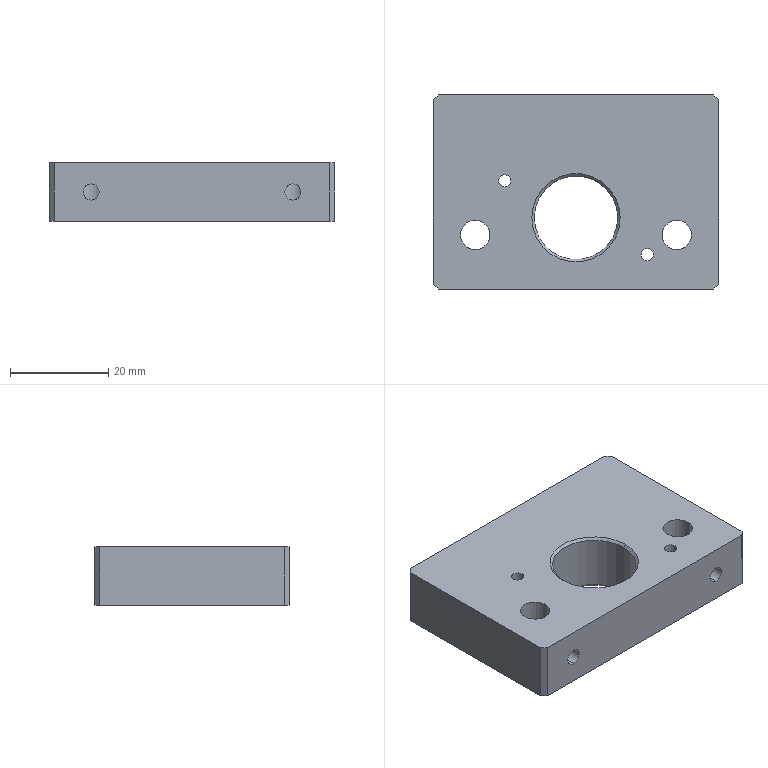Part | SolidWorks | features Chamfer 2, HoleWzd 2, Extrusion 1, MirrorPattern 1 | 1 solid | 36 faces | box 58 x 39.5 x 12 mm | volume 23617 mm3 | cylinder 18 | plane 10 | cone 8 | commonest cylinder face diameters 3.3 x8 2.5 x4 6 x4 17 x2
STEP:
#1=CARTESIAN_POINT('',(-8.5,-5.25,5.5));
#2=VERTEX_POINT('',#1);
#3=CARTESIAN_POINT('',(8.5,-5.25,5.5));
#4=VERTEX_POINT('',#3);
#5=CARTESIAN_POINT('',(0.,-5.25,5.5));
#6=DIRECTION('',(0.,0.,1.));
#7=DIRECTION('',(1.,0.,0.));
#8=AXIS2_PLACEMENT_3D('',#5,#6,#7);
#9=CIRCLE('',#8,8.5);
#10=EDGE_CURVE('',#2,#4,#9,.T.);
#11=ORIENTED_EDGE('',*,*,#10,.F.);
#12=CARTESIAN_POINT('',(-9.,-5.25,6.));
#13=VERTEX_POINT('',#12);
#14=CARTESIAN_POINT('',(-8.5,-5.25,5.5));
#15=DIRECTION('',(-0.7071,0.,0.7071));
#16=VECTOR('',#15,1000.);
#17=LINE('',#14,#16);
#18=EDGE_CURVE('',#2,#13,#17,.T.);
#19=ORIENTED_EDGE('',*,*,#18,.T.);
#20=CARTESIAN_POINT('',(9.,-5.25,6.));
#21=VERTEX_POINT('',#20);
#22=CARTESIAN_POINT('',(0.,-5.25,6.));
#23=DIRECTION('',(0.,0.,-1.));
#24=DIRECTION('',(1.,0.,0.));
#25=AXIS2_PLACEMENT_3D('',#22,#23,#24);
#26=CIRCLE('',#25,9.);
#27=EDGE_CURVE('',#21,#13,#26,.T.);
#28=ORIENTED_EDGE('',*,*,#27,.F.);
#29=CARTESIAN_POINT('',(8.5,-5.25,5.5));
#30=DIRECTION('',(0.7071,0.,0.7071));
#31=VECTOR('',#30,1000.);
#32=LINE('',#29,#31);
#33=EDGE_CURVE('',#4,#21,#32,.T.);
#34=ORIENTED_EDGE('',*,*,#33,.F.);
#35=EDGE_LOOP('',(#11,#19,#28,#34));
#36=FACE_OUTER_BOUND('',#35,.T.);
#37=CARTESIAN_POINT('',(0.,-5.25,5.5));
#38=DIRECTION('',(0.,0.,1.));
#39=DIRECTION('',(1.,0.,0.));
#40=AXIS2_PLACEMENT_3D('',#37,#38,#39);
#41=CONICAL_SURFACE('',#40,8.5,0.7854);
#42=ADVANCED_FACE('',(#36),#41,.F.);
#43=CARTESIAN_POINT('',(8.5,-5.25,-5.5));
#44=VERTEX_POINT('',#43);
#45=CARTESIAN_POINT('',(-8.5,-5.25,-5.5));
#46=VERTEX_POINT('',#45);
#47=CARTESIAN_POINT('',(0.,-5.25,-5.5));
#48=DIRECTION('',(0.,0.,-1.));
#49=DIRECTION('',(1.,0.,0.));
#50=AXIS2_PLACEMENT_3D('',#47,#48,#49);
#51=CIRCLE('',#50,8.5);
#52=EDGE_CURVE('',#44,#46,#51,.T.);
#53=ORIENTED_EDGE('',*,*,#52,.F.);
#54=CARTESIAN_POINT('',(9.,-5.25,-6.));
#55=VERTEX_POINT('',#54);
#56=CARTESIAN_POINT('',(9.,-5.25,-6.));
#57=DIRECTION('',(0.7071,0.,-0.7071));
#58=VECTOR('',#57,1000.);
#59=LINE('',#56,#58);
#60=EDGE_CURVE('',#44,#55,#59,.T.);
#61=ORIENTED_EDGE('',*,*,#60,.T.);
#62=CARTESIAN_POINT('',(-9.,-5.25,-6.));
#63=VERTEX_POINT('',#62);
#64=CARTESIAN_POINT('',(0.,-5.25,-6.));
#65=DIRECTION('',(0.,0.,1.));
#66=DIRECTION('',(1.,0.,0.));
#67=AXIS2_PLACEMENT_3D('',#64,#65,#66);
#68=CIRCLE('',#67,9.);
#69=EDGE_CURVE('',#63,#55,#68,.T.);
#70=ORIENTED_EDGE('',*,*,#69,.F.);
#71=CARTESIAN_POINT('',(-9.,-5.25,-6.));
#72=DIRECTION('',(-0.7071,0.,-0.7071));
#73=VECTOR('',#72,1000.);
#74=LINE('',#71,#73);
#75=EDGE_CURVE('',#46,#63,#74,.T.);
#76=ORIENTED_EDGE('',*,*,#75,.F.);
#77=EDGE_LOOP('',(#53,#61,#70,#76));
#78=FACE_OUTER_BOUND('',#77,.T.);
#79=CARTESIAN_POINT('',(0.,-5.25,-6.));
#80=DIRECTION('',(0.,0.,-1.));
#81=DIRECTION('',(-1.,0.,0.));
#82=AXIS2_PLACEMENT_3D('',#79,#80,#81);
#83=CONICAL_SURFACE('',#82,9.,0.7854);
#84=ADVANCED_FACE('',(#78),#83,.F.);
#85=CARTESIAN_POINT('',(-20.5,9.65,-1.65));
#86=VERTEX_POINT('',#85);
#87=CARTESIAN_POINT('',(-20.5,9.65,1.65));
#88=VERTEX_POINT('',#87);
#89=CARTESIAN_POINT('',(-20.5,9.65,0.));
#90=DIRECTION('',(0.,1.,0.));
#91=DIRECTION('',(0.,0.,1.));
#92=AXIS2_PLACEMENT_3D('',#89,#90,#91);
#93=CIRCLE('',#92,1.65);
#94=EDGE_CURVE('',#86,#88,#93,.T.);
#95=ORIENTED_EDGE('',*,*,#94,.F.);
#96=CARTESIAN_POINT('',(-20.5,19.75,-1.65));
#97=VERTEX_POINT('',#96);
#98=CARTESIAN_POINT('',(-20.5,19.75,-1.65));
#99=DIRECTION('',(0.,1.,0.));
#100=VECTOR('',#99,1000.);
#101=LINE('',#98,#100);
#102=EDGE_CURVE('',#86,#97,#101,.T.);
#103=ORIENTED_EDGE('',*,*,#102,.T.);
#104=CARTESIAN_POINT('',(-20.5,19.75,1.65));
#105=VERTEX_POINT('',#104);
#106=CARTESIAN_POINT('',(-20.5,19.75,0.));
#107=DIRECTION('',(0.,1.,0.));
#108=DIRECTION('',(0.,0.,1.));
#109=AXIS2_PLACEMENT_3D('',#106,#107,#108);
#110=CIRCLE('',#109,1.65);
#111=EDGE_CURVE('',#97,#105,#110,.T.);
#112=ORIENTED_EDGE('',*,*,#111,.T.);
#113=CARTESIAN_POINT('',(-20.5,19.75,1.65));
#114=DIRECTION('',(0.,1.,0.));
#115=VECTOR('',#114,1000.);
#116=LINE('',#113,#115);
#117=EDGE_CURVE('',#88,#105,#116,.T.);
#118=ORIENTED_EDGE('',*,*,#117,.F.);
#119=EDGE_LOOP('',(#95,#103,#112,#118));
#120=FACE_OUTER_BOUND('',#119,.T.);
#121=CARTESIAN_POINT('',(-20.5,19.75,0.));
#122=DIRECTION('',(0.,1.,0.));
#123=DIRECTION('',(0.,0.,1.));
#124=AXIS2_PLACEMENT_3D('',#121,#122,#123);
#125=CYLINDRICAL_SURFACE('',#124,1.65);
#126=ADVANCED_FACE('',(#120),#125,.F.);
#127=CARTESIAN_POINT('',(-20.5,8.659,0.));
#128=VERTEX_POINT('',#127);
#129=CARTESIAN_POINT('',(-20.5,9.65,1.65));
#130=DIRECTION('',(0.,0.515,0.8572));
#131=VECTOR('',#130,1000.);
#132=LINE('',#129,#131);
#133=EDGE_CURVE('',#128,#88,#132,.T.);
#134=ORIENTED_EDGE('',*,*,#133,.F.);
#135=CARTESIAN_POINT('',(-20.5,9.65,-1.65));
#136=DIRECTION('',(0.,0.515,-0.8572));
#137=VECTOR('',#136,1000.);
#138=LINE('',#135,#137);
#139=EDGE_CURVE('',#128,#86,#138,.T.);
#140=ORIENTED_EDGE('',*,*,#139,.T.);
#141=ORIENTED_EDGE('',*,*,#94,.T.);
#142=EDGE_LOOP('',(#134,#140,#141));
#143=FACE_OUTER_BOUND('',#142,.T.);
#144=CARTESIAN_POINT('',(-20.5,9.65,0.));
#145=DIRECTION('',(0.,1.,0.));
#146=DIRECTION('',(0.,0.,1.));
#147=AXIS2_PLACEMENT_3D('',#144,#145,#146);
#148=CONICAL_SURFACE('',#147,1.65,1.03);
#149=ADVANCED_FACE('',(#143),#148,.F.);
#150=CARTESIAN_POINT('',(20.5,9.65,-1.65));
#151=VERTEX_POINT('',#150);
#152=CARTESIAN_POINT('',(20.5,9.65,1.65));
#153=VERTEX_POINT('',#152);
#154=CARTESIAN_POINT('',(20.5,9.65,0.));
#155=DIRECTION('',(0.,1.,0.));
#156=DIRECTION('',(0.,0.,1.));
#157=AXIS2_PLACEMENT_3D('',#154,#155,#156);
#158=CIRCLE('',#157,1.65);
#159=EDGE_CURVE('',#151,#153,#158,.T.);
#160=ORIENTED_EDGE('',*,*,#159,.F.);
#161=CARTESIAN_POINT('',(20.5,19.75,-1.65));
#162=VERTEX_POINT('',#161);
#163=CARTESIAN_POINT('',(20.5,19.75,-1.65));
#164=DIRECTION('',(0.,1.,0.));
#165=VECTOR('',#164,1000.);
#166=LINE('',#163,#165);
#167=EDGE_CURVE('',#151,#162,#166,.T.);
#168=ORIENTED_EDGE('',*,*,#167,.T.);
#169=CARTESIAN_POINT('',(20.5,19.75,1.65));
#170=VERTEX_POINT('',#169);
#171=CARTESIAN_POINT('',(20.5,19.75,0.));
#172=DIRECTION('',(0.,1.,0.));
#173=DIRECTION('',(0.,0.,1.));
#174=AXIS2_PLACEMENT_3D('',#171,#172,#173);
#175=CIRCLE('',#174,1.65);
#176=EDGE_CURVE('',#162,#170,#175,.T.);
#177=ORIENTED_EDGE('',*,*,#176,.T.);
#178=CARTESIAN_POINT('',(20.5,19.75,1.65));
#179=DIRECTION('',(0.,1.,0.));
#180=VECTOR('',#179,1000.);
#181=LINE('',#178,#180);
#182=EDGE_CURVE('',#153,#170,#181,.T.);
#183=ORIENTED_EDGE('',*,*,#182,.F.);
#184=EDGE_LOOP('',(#160,#168,#177,#183));
#185=FACE_OUTER_BOUND('',#184,.T.);
#186=CARTESIAN_POINT('',(20.5,19.75,0.));
#187=DIRECTION('',(0.,1.,0.));
#188=DIRECTION('',(0.,0.,1.));
#189=AXIS2_PLACEMENT_3D('',#186,#187,#188);
#190=CYLINDRICAL_SURFACE('',#189,1.65);
#191=ADVANCED_FACE('',(#185),#190,.F.);
#192=CARTESIAN_POINT('',(20.5,8.659,0.));
#193=VERTEX_POINT('',#192);
#194=CARTESIAN_POINT('',(20.5,9.65,1.65));
#195=DIRECTION('',(0.,0.515,0.8572));
#196=VECTOR('',#195,1000.);
#197=LINE('',#194,#196);
#198=EDGE_CURVE('',#193,#153,#197,.T.);
#199=ORIENTED_EDGE('',*,*,#198,.F.);
#200=CARTESIAN_POINT('',(20.5,9.65,-1.65));
#201=DIRECTION('',(0.,0.515,-0.8572));
#202=VECTOR('',#201,1000.);
#203=LINE('',#200,#202);
#204=EDGE_CURVE('',#193,#151,#203,.T.);
#205=ORIENTED_EDGE('',*,*,#204,.T.);
#206=ORIENTED_EDGE('',*,*,#159,.T.);
#207=EDGE_LOOP('',(#199,#205,#206));
#208=FACE_OUTER_BOUND('',#207,.T.);
#209=CARTESIAN_POINT('',(20.5,9.65,0.));
#210=DIRECTION('',(0.,1.,0.));
#211=DIRECTION('',(0.,0.,1.));
#212=AXIS2_PLACEMENT_3D('',#209,#210,#211);
#213=CONICAL_SURFACE('',#212,1.65,1.03);
#214=ADVANCED_FACE('',(#208),#213,.F.);
#215=CARTESIAN_POINT('',(-20.5,-11.75,-1.65));
#216=VERTEX_POINT('',#215);
#217=CARTESIAN_POINT('',(-20.5,-11.75,1.65));
#218=VERTEX_POINT('',#217);
#219=CARTESIAN_POINT('',(-20.5,-11.75,-1.65));
#220=CARTESIAN_POINT('',(-20.612,-11.75,-1.65));
#221=CARTESIAN_POINT('',(-20.721,-11.744,-1.639));
#222=CARTESIAN_POINT('',(-20.935,-11.72,-1.595));
#223=CARTESIAN_POINT('',(-21.041,-11.703,-1.563));
#224=CARTESIAN_POINT('',(-21.34,-11.637,-1.437));
#225=CARTESIAN_POINT('',(-21.52,-11.576,-1.314));
#226=CARTESIAN_POINT('',(-21.817,-11.45,-1.016));
#227=CARTESIAN_POINT('',(-21.938,-11.385,-0.8367));
#228=CARTESIAN_POINT('',(-22.063,-11.311,-0.5406));
#229=CARTESIAN_POINT('',(-22.095,-11.291,-0.4349));
#230=CARTESIAN_POINT('',(-22.139,-11.263,-0.2211));
#231=CARTESIAN_POINT('',(-22.15,-11.256,-0.1125));
#232=CARTESIAN_POINT('',(-22.15,-11.255,0.1082));
#233=CARTESIAN_POINT('',(-22.139,-11.263,0.2198));
#234=CARTESIAN_POINT('',(-22.096,-11.291,0.434));
#235=CARTESIAN_POINT('',(-22.063,-11.311,0.5391));
#236=CARTESIAN_POINT('',(-21.938,-11.385,0.8379));
#237=CARTESIAN_POINT('',(-21.816,-11.451,1.017));
#238=CARTESIAN_POINT('',(-21.518,-11.576,1.315));
#239=CARTESIAN_POINT('',(-21.338,-11.638,1.438));
#240=CARTESIAN_POINT('',(-21.041,-11.703,1.563));
#241=CARTESIAN_POINT('',(-20.935,-11.72,1.595));
#242=CARTESIAN_POINT('',(-20.719,-11.744,1.639));
#243=CARTESIAN_POINT('',(-20.61,-11.75,1.65));
#244=CARTESIAN_POINT('',(-20.5,-11.75,1.65));
#245=B_SPLINE_CURVE_WITH_KNOTS('',3,(#219,#220,#221,#222,#223,#224,#225,#226,#227,#228,#229,#230,#231,#232,#233,#234,#235,#236,#237,#238,#239,#240,#241,#242,#243,#244),.UNSPECIFIED.,.F.,.F.,(4,2,2,2,2,2,2,2,2,2,2,2,4),(0.,0.0003294,0.0006588,0.001318,0.001976,0.002306,0.002635,0.002965,0.003294,0.003953,0.004612,0.004941,0.00527),.UNSPECIFIED.);
#246=EDGE_CURVE('',#216,#218,#245,.T.);
#247=ORIENTED_EDGE('',*,*,#246,.T.);
#248=CARTESIAN_POINT('',(-20.5,-19.75,1.65));
#249=VERTEX_POINT('',#248);
#250=CARTESIAN_POINT('',(-20.5,-19.75,1.65));
#251=DIRECTION('',(0.,-1.,0.));
#252=VECTOR('',#251,1000.);
#253=LINE('',#250,#252);
#254=EDGE_CURVE('',#218,#249,#253,.T.);
#255=ORIENTED_EDGE('',*,*,#254,.T.);
#256=CARTESIAN_POINT('',(-20.5,-19.75,-1.65));
#257=VERTEX_POINT('',#256);
#258=CARTESIAN_POINT('',(-20.5,-19.75,0.));
#259=DIRECTION('',(0.,-1.,0.));
#260=DIRECTION('',(0.,0.,-1.));
#261=AXIS2_PLACEMENT_3D('',#258,#259,#260);
#262=CIRCLE('',#261,1.65);
#263=EDGE_CURVE('',#249,#257,#262,.T.);
#264=ORIENTED_EDGE('',*,*,#263,.T.);
#265=CARTESIAN_POINT('',(-20.5,-19.75,-1.65));
#266=DIRECTION('',(0.,-1.,0.));
#267=VECTOR('',#266,1000.);
#268=LINE('',#265,#267);
#269=EDGE_CURVE('',#216,#257,#268,.T.);
#270=ORIENTED_EDGE('',*,*,#269,.F.);
#271=EDGE_LOOP('',(#247,#255,#264,#270));
#272=FACE_OUTER_BOUND('',#271,.T.);
#273=CARTESIAN_POINT('',(-20.5,-19.75,0.));
#274=DIRECTION('',(0.,-1.,0.));
#275=DIRECTION('',(0.,0.,-1.));
#276=AXIS2_PLACEMENT_3D('',#273,#274,#275);
#277=CYLINDRICAL_SURFACE('',#276,1.65);
#278=ADVANCED_FACE('',(#272),#277,.F.);
#279=CARTESIAN_POINT('',(20.5,-11.75,-1.65));
#280=VERTEX_POINT('',#279);
#281=CARTESIAN_POINT('',(20.5,-11.75,1.65));
#282=VERTEX_POINT('',#281);
#283=CARTESIAN_POINT('',(20.5,-11.75,-1.65));
#284=CARTESIAN_POINT('',(20.388,-11.75,-1.65));
#285=CARTESIAN_POINT('',(20.279,-11.744,-1.639));
#286=CARTESIAN_POINT('',(20.065,-11.72,-1.595));
#287=CARTESIAN_POINT('',(19.959,-11.703,-1.563));
#288=CARTESIAN_POINT('',(19.66,-11.637,-1.437));
#289=CARTESIAN_POINT('',(19.48,-11.576,-1.314));
#290=CARTESIAN_POINT('',(19.183,-11.45,-1.016));
#291=CARTESIAN_POINT('',(19.062,-11.385,-0.8367));
#292=CARTESIAN_POINT('',(18.937,-11.311,-0.5406));
#293=CARTESIAN_POINT('',(18.905,-11.291,-0.4349));
#294=CARTESIAN_POINT('',(18.861,-11.263,-0.2211));
#295=CARTESIAN_POINT('',(18.85,-11.256,-0.1125));
#296=CARTESIAN_POINT('',(18.85,-11.255,0.1082));
#297=CARTESIAN_POINT('',(18.861,-11.263,0.2198));
#298=CARTESIAN_POINT('',(18.904,-11.291,0.434));
#299=CARTESIAN_POINT('',(18.937,-11.311,0.5391));
#300=CARTESIAN_POINT('',(19.062,-11.385,0.8379));
#301=CARTESIAN_POINT('',(19.184,-11.451,1.017));
#302=CARTESIAN_POINT('',(19.482,-11.576,1.315));
#303=CARTESIAN_POINT('',(19.662,-11.638,1.438));
#304=CARTESIAN_POINT('',(19.959,-11.703,1.563));
#305=CARTESIAN_POINT('',(20.065,-11.72,1.595));
#306=CARTESIAN_POINT('',(20.281,-11.744,1.639));
#307=CARTESIAN_POINT('',(20.39,-11.75,1.65));
#308=CARTESIAN_POINT('',(20.5,-11.75,1.65));
#309=B_SPLINE_CURVE_WITH_KNOTS('',3,(#283,#284,#285,#286,#287,#288,#289,#290,#291,#292,#293,#294,#295,#296,#297,#298,#299,#300,#301,#302,#303,#304,#305,#306,#307,#308),.UNSPECIFIED.,.F.,.F.,(4,2,2,2,2,2,2,2,2,2,2,2,4),(0.,0.0003294,0.0006588,0.001318,0.001976,0.002306,0.002635,0.002965,0.003294,0.003953,0.004612,0.004941,0.00527),.UNSPECIFIED.);
#310=EDGE_CURVE('',#280,#282,#309,.T.);
#311=ORIENTED_EDGE('',*,*,#310,.T.);
#312=CARTESIAN_POINT('',(20.5,-19.75,1.65));
#313=VERTEX_POINT('',#312);
#314=CARTESIAN_POINT('',(20.5,-19.75,1.65));
#315=DIRECTION('',(0.,-1.,0.));
#316=VECTOR('',#315,1000.);
#317=LINE('',#314,#316);
#318=EDGE_CURVE('',#282,#313,#317,.T.);
#319=ORIENTED_EDGE('',*,*,#318,.T.);
#320=CARTESIAN_POINT('',(20.5,-19.75,-1.65));
#321=VERTEX_POINT('',#320);
#322=CARTESIAN_POINT('',(20.5,-19.75,0.));
#323=DIRECTION('',(0.,-1.,0.));
#324=DIRECTION('',(0.,0.,-1.));
#325=AXIS2_PLACEMENT_3D('',#322,#323,#324);
#326=CIRCLE('',#325,1.65);
#327=EDGE_CURVE('',#313,#321,#326,.T.);
#328=ORIENTED_EDGE('',*,*,#327,.T.);
#329=CARTESIAN_POINT('',(20.5,-19.75,-1.65));
#330=DIRECTION('',(0.,-1.,0.));
#331=VECTOR('',#330,1000.);
#332=LINE('',#329,#331);
#333=EDGE_CURVE('',#280,#321,#332,.T.);
#334=ORIENTED_EDGE('',*,*,#333,.F.);
#335=EDGE_LOOP('',(#311,#319,#328,#334));
#336=FACE_OUTER_BOUND('',#335,.T.);
#337=CARTESIAN_POINT('',(20.5,-19.75,0.));
#338=DIRECTION('',(0.,-1.,0.));
#339=DIRECTION('',(0.,0.,-1.));
#340=AXIS2_PLACEMENT_3D('',#337,#338,#339);
#341=CYLINDRICAL_SURFACE('',#340,1.65);
#342=ADVANCED_FACE('',(#336),#341,.F.);
#343=CARTESIAN_POINT('',(-15.75,2.25,-6.));
#344=VERTEX_POINT('',#343);
#345=CARTESIAN_POINT('',(-13.25,2.25,-6.));
#346=VERTEX_POINT('',#345);
#347=CARTESIAN_POINT('',(-14.5,2.25,-6.));
#348=DIRECTION('',(0.,0.,1.));
#349=DIRECTION('',(1.,0.,0.));
#350=AXIS2_PLACEMENT_3D('',#347,#348,#349);
#351=CIRCLE('',#350,1.25);
#352=EDGE_CURVE('',#344,#346,#351,.T.);
#353=ORIENTED_EDGE('',*,*,#352,.F.);
#354=CARTESIAN_POINT('',(-15.75,2.25,6.));
#355=VERTEX_POINT('',#354);
#356=CARTESIAN_POINT('',(-15.75,2.25,6.));
#357=DIRECTION('',(0.,0.,1.));
#358=VECTOR('',#357,1000.);
#359=LINE('',#356,#358);
#360=EDGE_CURVE('',#344,#355,#359,.T.);
#361=ORIENTED_EDGE('',*,*,#360,.T.);
#362=CARTESIAN_POINT('',(-13.25,2.25,6.));
#363=VERTEX_POINT('',#362);
#364=CARTESIAN_POINT('',(-14.5,2.25,6.));
#365=DIRECTION('',(0.,0.,1.));
#366=DIRECTION('',(1.,0.,0.));
#367=AXIS2_PLACEMENT_3D('',#364,#365,#366);
#368=CIRCLE('',#367,1.25);
#369=EDGE_CURVE('',#355,#363,#368,.T.);
#370=ORIENTED_EDGE('',*,*,#369,.T.);
#371=CARTESIAN_POINT('',(-13.25,2.25,6.));
#372=DIRECTION('',(0.,0.,1.));
#373=VECTOR('',#372,1000.);
#374=LINE('',#371,#373);
#375=EDGE_CURVE('',#346,#363,#374,.T.);
#376=ORIENTED_EDGE('',*,*,#375,.F.);
#377=EDGE_LOOP('',(#353,#361,#370,#376));
#378=FACE_OUTER_BOUND('',#377,.T.);
#379=CARTESIAN_POINT('',(-14.5,2.25,6.));
#380=DIRECTION('',(0.,0.,1.));
#381=DIRECTION('',(1.,0.,0.));
#382=AXIS2_PLACEMENT_3D('',#379,#380,#381);
#383=CYLINDRICAL_SURFACE('',#382,1.25);
#384=ADVANCED_FACE('',(#378),#383,.F.);
#385=CARTESIAN_POINT('',(13.25,-12.75,-6.));
#386=VERTEX_POINT('',#385);
#387=CARTESIAN_POINT('',(15.75,-12.75,-6.));
#388=VERTEX_POINT('',#387);
#389=CARTESIAN_POINT('',(14.5,-12.75,-6.));
#390=DIRECTION('',(0.,0.,1.));
#391=DIRECTION('',(1.,0.,0.));
#392=AXIS2_PLACEMENT_3D('',#389,#390,#391);
#393=CIRCLE('',#392,1.25);
#394=EDGE_CURVE('',#386,#388,#393,.T.);
#395=ORIENTED_EDGE('',*,*,#394,.F.);
#396=CARTESIAN_POINT('',(13.25,-12.75,6.));
#397=VERTEX_POINT('',#396);
#398=CARTESIAN_POINT('',(13.25,-12.75,6.));
#399=DIRECTION('',(0.,0.,1.));
#400=VECTOR('',#399,1000.);
#401=LINE('',#398,#400);
#402=EDGE_CURVE('',#386,#397,#401,.T.);
#403=ORIENTED_EDGE('',*,*,#402,.T.);
#404=CARTESIAN_POINT('',(15.75,-12.75,6.));
#405=VERTEX_POINT('',#404);
#406=CARTESIAN_POINT('',(14.5,-12.75,6.));
#407=DIRECTION('',(0.,0.,1.));
#408=DIRECTION('',(1.,0.,0.));
#409=AXIS2_PLACEMENT_3D('',#406,#407,#408);
#410=CIRCLE('',#409,1.25);
#411=EDGE_CURVE('',#397,#405,#410,.T.);
#412=ORIENTED_EDGE('',*,*,#411,.T.);
#413=CARTESIAN_POINT('',(15.75,-12.75,6.));
#414=DIRECTION('',(0.,0.,1.));
#415=VECTOR('',#414,1000.);
#416=LINE('',#413,#415);
#417=EDGE_CURVE('',#388,#405,#416,.T.);
#418=ORIENTED_EDGE('',*,*,#417,.F.);
#419=EDGE_LOOP('',(#395,#403,#412,#418));
#420=FACE_OUTER_BOUND('',#419,.T.);
#421=CARTESIAN_POINT('',(14.5,-12.75,6.));
#422=DIRECTION('',(0.,0.,1.));
#423=DIRECTION('',(1.,0.,0.));
#424=AXIS2_PLACEMENT_3D('',#421,#422,#423);
#425=CYLINDRICAL_SURFACE('',#424,1.25);
#426=ADVANCED_FACE('',(#420),#425,.F.);
#427=ORIENTED_EDGE('',*,*,#310,.F.);
#428=CARTESIAN_POINT('',(20.5,-11.75,1.65));
#429=CARTESIAN_POINT('',(20.61,-11.75,1.65));
#430=CARTESIAN_POINT('',(20.722,-11.744,1.639));
#431=CARTESIAN_POINT('',(20.936,-11.72,1.595));
#432=CARTESIAN_POINT('',(21.041,-11.703,1.563));
#433=CARTESIAN_POINT('',(21.241,-11.659,1.478));
#434=CARTESIAN_POINT('',(21.335,-11.633,1.427));
#435=CARTESIAN_POINT('',(21.512,-11.576,1.308));
#436=CARTESIAN_POINT('',(21.594,-11.544,1.239));
#437=CARTESIAN_POINT('',(21.818,-11.45,1.015));
#438=CARTESIAN_POINT('',(21.938,-11.384,0.836));
#439=CARTESIAN_POINT('',(22.104,-11.287,0.4427));
#440=CARTESIAN_POINT('',(22.15,-11.256,0.222));
#441=CARTESIAN_POINT('',(22.15,-11.255,-0.1068));
#442=CARTESIAN_POINT('',(22.139,-11.263,-0.2187));
#443=CARTESIAN_POINT('',(22.096,-11.29,-0.4332));
#444=CARTESIAN_POINT('',(22.064,-11.311,-0.5369));
#445=CARTESIAN_POINT('',(21.98,-11.36,-0.7373));
#446=CARTESIAN_POINT('',(21.929,-11.388,-0.831));
#447=CARTESIAN_POINT('',(21.811,-11.449,-1.007));
#448=CARTESIAN_POINT('',(21.743,-11.482,-1.09));
#449=CARTESIAN_POINT('',(21.594,-11.545,-1.24));
#450=CARTESIAN_POINT('',(21.513,-11.575,-1.307));
#451=CARTESIAN_POINT('',(21.336,-11.633,-1.427));
#452=CARTESIAN_POINT('',(21.24,-11.659,-1.478));
#453=CARTESIAN_POINT('',(20.943,-11.724,-1.604));
#454=CARTESIAN_POINT('',(20.723,-11.75,-1.65));
#455=CARTESIAN_POINT('',(20.5,-11.75,-1.65));
#456=B_SPLINE_CURVE_WITH_KNOTS('',3,(#428,#429,#430,#431,#432,#433,#434,#435,#436,#437,#438,#439,#440,#441,#442,#443,#444,#445,#446,#447,#448,#449,#450,#451,#452,#453,#454,#455),.UNSPECIFIED.,.F.,.F.,(4,2,2,2,2,2,2,2,2,2,2,2,2,4),(0.00527,0.005599,0.005928,0.006256,0.006585,0.007242,0.007899,0.008228,0.008556,0.008885,0.009213,0.009542,0.009871,0.01053),.UNSPECIFIED.);
#457=EDGE_CURVE('',#282,#280,#456,.T.);
#458=ORIENTED_EDGE('',*,*,#457,.F.);
#459=EDGE_LOOP('',(#427,#458));
#460=FACE_BOUND('',#459,.T.);
#461=CARTESIAN_POINT('',(17.5,-8.75,6.));
#462=VERTEX_POINT('',#461);
#463=CARTESIAN_POINT('',(23.5,-8.75,6.));
#464=VERTEX_POINT('',#463);
#465=CARTESIAN_POINT('',(20.5,-8.75,6.));
#466=DIRECTION('',(0.,0.,1.));
#467=DIRECTION('',(1.,0.,0.));
#468=AXIS2_PLACEMENT_3D('',#465,#466,#467);
#469=CIRCLE('',#468,3.);
#470=EDGE_CURVE('',#462,#464,#469,.T.);
#471=ORIENTED_EDGE('',*,*,#470,.T.);
#472=CARTESIAN_POINT('',(23.5,-8.75,-6.));
#473=VERTEX_POINT('',#472);
#474=CARTESIAN_POINT('',(23.5,-8.75,6.));
#475=DIRECTION('',(0.,0.,-1.));
#476=VECTOR('',#475,1000.);
#477=LINE('',#474,#476);
#478=EDGE_CURVE('',#464,#473,#477,.T.);
#479=ORIENTED_EDGE('',*,*,#478,.T.);
#480=CARTESIAN_POINT('',(17.5,-8.75,-6.));
#481=VERTEX_POINT('',#480);
#482=CARTESIAN_POINT('',(20.5,-8.75,-6.));
#483=DIRECTION('',(0.,0.,1.));
#484=DIRECTION('',(1.,0.,0.));
#485=AXIS2_PLACEMENT_3D('',#482,#483,#484);
#486=CIRCLE('',#485,3.);
#487=EDGE_CURVE('',#481,#473,#486,.T.);
#488=ORIENTED_EDGE('',*,*,#487,.F.);
#489=CARTESIAN_POINT('',(17.5,-8.75,6.));
#490=DIRECTION('',(0.,0.,-1.));
#491=VECTOR('',#490,1000.);
#492=LINE('',#489,#491);
#493=EDGE_CURVE('',#462,#481,#492,.T.);
#494=ORIENTED_EDGE('',*,*,#493,.F.);
#495=EDGE_LOOP('',(#471,#479,#488,#494));
#496=FACE_OUTER_BOUND('',#495,.T.);
#497=CARTESIAN_POINT('',(20.5,-8.75,6.));
#498=DIRECTION('',(0.,0.,-1.));
#499=DIRECTION('',(-1.,0.,0.));
#500=AXIS2_PLACEMENT_3D('',#497,#498,#499);
#501=CYLINDRICAL_SURFACE('',#500,3.);
#502=ADVANCED_FACE('',(#460,#496),#501,.F.);
#503=ORIENTED_EDGE('',*,*,#246,.F.);
#504=CARTESIAN_POINT('',(-20.5,-11.75,1.65));
#505=CARTESIAN_POINT('',(-20.39,-11.75,1.65));
#506=CARTESIAN_POINT('',(-20.278,-11.744,1.639));
#507=CARTESIAN_POINT('',(-20.064,-11.72,1.595));
#508=CARTESIAN_POINT('',(-19.959,-11.703,1.563));
#509=CARTESIAN_POINT('',(-19.759,-11.659,1.478));
#510=CARTESIAN_POINT('',(-19.665,-11.633,1.427));
#511=CARTESIAN_POINT('',(-19.488,-11.576,1.308));
#512=CARTESIAN_POINT('',(-19.406,-11.544,1.239));
#513=CARTESIAN_POINT('',(-19.182,-11.45,1.015));
#514=CARTESIAN_POINT('',(-19.062,-11.384,0.836));
#515=CARTESIAN_POINT('',(-18.896,-11.287,0.4427));
#516=CARTESIAN_POINT('',(-18.85,-11.256,0.222));
#517=CARTESIAN_POINT('',(-18.85,-11.255,-0.1068));
#518=CARTESIAN_POINT('',(-18.861,-11.263,-0.2187));
#519=CARTESIAN_POINT('',(-18.904,-11.29,-0.4332));
#520=CARTESIAN_POINT('',(-18.936,-11.311,-0.5369));
#521=CARTESIAN_POINT('',(-19.02,-11.36,-0.7373));
#522=CARTESIAN_POINT('',(-19.071,-11.388,-0.831));
#523=CARTESIAN_POINT('',(-19.189,-11.449,-1.007));
#524=CARTESIAN_POINT('',(-19.257,-11.482,-1.09));
#525=CARTESIAN_POINT('',(-19.406,-11.545,-1.24));
#526=CARTESIAN_POINT('',(-19.487,-11.575,-1.307));
#527=CARTESIAN_POINT('',(-19.664,-11.633,-1.427));
#528=CARTESIAN_POINT('',(-19.76,-11.659,-1.478));
#529=CARTESIAN_POINT('',(-20.057,-11.724,-1.604));
#530=CARTESIAN_POINT('',(-20.277,-11.75,-1.65));
#531=CARTESIAN_POINT('',(-20.5,-11.75,-1.65));
#532=B_SPLINE_CURVE_WITH_KNOTS('',3,(#504,#505,#506,#507,#508,#509,#510,#511,#512,#513,#514,#515,#516,#517,#518,#519,#520,#521,#522,#523,#524,#525,#526,#527,#528,#529,#530,#531),.UNSPECIFIED.,.F.,.F.,(4,2,2,2,2,2,2,2,2,2,2,2,2,4),(0.00527,0.005599,0.005928,0.006256,0.006585,0.007242,0.007899,0.008228,0.008556,0.008885,0.009213,0.009542,0.009871,0.01053),.UNSPECIFIED.);
#533=EDGE_CURVE('',#218,#216,#532,.T.);
#534=ORIENTED_EDGE('',*,*,#533,.F.);
#535=EDGE_LOOP('',(#503,#534));
#536=FACE_BOUND('',#535,.T.);
#537=CARTESIAN_POINT('',(-23.5,-8.75,6.));
#538=VERTEX_POINT('',#537);
#539=CARTESIAN_POINT('',(-17.5,-8.75,6.));
#540=VERTEX_POINT('',#539);
#541=CARTESIAN_POINT('',(-20.5,-8.75,6.));
#542=DIRECTION('',(0.,0.,1.));
#543=DIRECTION('',(1.,0.,0.));
#544=AXIS2_PLACEMENT_3D('',#541,#542,#543);
#545=CIRCLE('',#544,3.);
#546=EDGE_CURVE('',#538,#540,#545,.T.);
#547=ORIENTED_EDGE('',*,*,#546,.T.);
#548=CARTESIAN_POINT('',(-17.5,-8.75,-6.));
#549=VERTEX_POINT('',#548);
#550=CARTESIAN_POINT('',(-17.5,-8.75,6.));
#551=DIRECTION('',(0.,0.,-1.));
#552=VECTOR('',#551,1000.);
#553=LINE('',#550,#552);
#554=EDGE_CURVE('',#540,#549,#553,.T.);
#555=ORIENTED_EDGE('',*,*,#554,.T.);
#556=CARTESIAN_POINT('',(-23.5,-8.75,-6.));
#557=VERTEX_POINT('',#556);
#558=CARTESIAN_POINT('',(-20.5,-8.75,-6.));
#559=DIRECTION('',(0.,0.,1.));
#560=DIRECTION('',(1.,0.,0.));
#561=AXIS2_PLACEMENT_3D('',#558,#559,#560);
#562=CIRCLE('',#561,3.);
#563=EDGE_CURVE('',#557,#549,#562,.T.);
#564=ORIENTED_EDGE('',*,*,#563,.F.);
#565=CARTESIAN_POINT('',(-23.5,-8.75,6.));
#566=DIRECTION('',(0.,0.,-1.));
#567=VECTOR('',#566,1000.);
#568=LINE('',#565,#567);
#569=EDGE_CURVE('',#538,#557,#568,.T.);
#570=ORIENTED_EDGE('',*,*,#569,.F.);
#571=EDGE_LOOP('',(#547,#555,#564,#570));
#572=FACE_OUTER_BOUND('',#571,.T.);
#573=CARTESIAN_POINT('',(-20.5,-8.75,6.));
#574=DIRECTION('',(0.,0.,-1.));
#575=DIRECTION('',(-1.,0.,0.));
#576=AXIS2_PLACEMENT_3D('',#573,#574,#575);
#577=CYLINDRICAL_SURFACE('',#576,3.);
#578=ADVANCED_FACE('',(#536,#572),#577,.F.);
#579=ORIENTED_EDGE('',*,*,#10,.T.);
#580=CARTESIAN_POINT('',(8.5,-5.25,6.));
#581=DIRECTION('',(0.,0.,-1.));
#582=VECTOR('',#581,1000.);
#583=LINE('',#580,#582);
#584=EDGE_CURVE('',#4,#44,#583,.T.);
#585=ORIENTED_EDGE('',*,*,#584,.T.);
#586=ORIENTED_EDGE('',*,*,#52,.T.);
#587=CARTESIAN_POINT('',(-8.5,-5.25,6.));
#588=DIRECTION('',(0.,0.,-1.));
#589=VECTOR('',#588,1000.);
#590=LINE('',#587,#589);
#591=EDGE_CURVE('',#2,#46,#590,.T.);
#592=ORIENTED_EDGE('',*,*,#591,.F.);
#593=EDGE_LOOP('',(#579,#585,#586,#592));
#594=FACE_OUTER_BOUND('',#593,.T.);
#595=CARTESIAN_POINT('',(0.,-5.25,6.));
#596=DIRECTION('',(0.,0.,-1.));
#597=DIRECTION('',(-1.,0.,0.));
#598=AXIS2_PLACEMENT_3D('',#595,#596,#597);
#599=CYLINDRICAL_SURFACE('',#598,8.5);
#600=ADVANCED_FACE('',(#594),#599,.F.);
#601=ORIENTED_EDGE('',*,*,#27,.T.);
#602=CARTESIAN_POINT('',(0.,-5.25,6.));
#603=DIRECTION('',(0.,0.,-1.));
#604=DIRECTION('',(1.,0.,0.));
#605=AXIS2_PLACEMENT_3D('',#602,#603,#604);
#606=CIRCLE('',#605,9.);
#607=EDGE_CURVE('',#13,#21,#606,.T.);
#608=ORIENTED_EDGE('',*,*,#607,.T.);
#609=EDGE_LOOP('',(#601,#608));
#610=FACE_BOUND('',#609,.T.);
#611=CARTESIAN_POINT('',(-14.5,2.25,6.));
#612=DIRECTION('',(0.,0.,1.));
#613=DIRECTION('',(1.,0.,0.));
#614=AXIS2_PLACEMENT_3D('',#611,#612,#613);
#615=CIRCLE('',#614,1.25);
#616=EDGE_CURVE('',#363,#355,#615,.T.);
#617=ORIENTED_EDGE('',*,*,#616,.F.);
#618=ORIENTED_EDGE('',*,*,#369,.F.);
#619=EDGE_LOOP('',(#617,#618));
#620=FACE_BOUND('',#619,.T.);
#621=CARTESIAN_POINT('',(14.5,-12.75,6.));
#622=DIRECTION('',(0.,0.,1.));
#623=DIRECTION('',(1.,0.,0.));
#624=AXIS2_PLACEMENT_3D('',#621,#622,#623);
#625=CIRCLE('',#624,1.25);
#626=EDGE_CURVE('',#405,#397,#625,.T.);
#627=ORIENTED_EDGE('',*,*,#626,.F.);
#628=ORIENTED_EDGE('',*,*,#411,.F.);
#629=EDGE_LOOP('',(#627,#628));
#630=FACE_BOUND('',#629,.T.);
#631=ORIENTED_EDGE('',*,*,#546,.F.);
#632=CARTESIAN_POINT('',(-20.5,-8.75,6.));
#633=DIRECTION('',(0.,0.,1.));
#634=DIRECTION('',(1.,0.,0.));
#635=AXIS2_PLACEMENT_3D('',#632,#633,#634);
#636=CIRCLE('',#635,3.);
#637=EDGE_CURVE('',#540,#538,#636,.T.);
#638=ORIENTED_EDGE('',*,*,#637,.F.);
#639=EDGE_LOOP('',(#631,#638));
#640=FACE_BOUND('',#639,.T.);
#641=CARTESIAN_POINT('',(29.,-18.75,6.));
#642=VERTEX_POINT('',#641);
#643=CARTESIAN_POINT('',(29.,18.75,6.));
#644=VERTEX_POINT('',#643);
#645=CARTESIAN_POINT('',(29.,19.75,6.));
#646=DIRECTION('',(0.,1.,0.));
#647=VECTOR('',#646,1000.);
#648=LINE('',#645,#647);
#649=EDGE_CURVE('',#642,#644,#648,.T.);
#650=ORIENTED_EDGE('',*,*,#649,.T.);
#651=CARTESIAN_POINT('',(28.,19.75,6.));
#652=VERTEX_POINT('',#651);
#653=CARTESIAN_POINT('',(48.25,-0.5,6.));
#654=DIRECTION('',(-0.7071,0.7071,0.));
#655=VECTOR('',#654,1000.);
#656=LINE('',#653,#655);
#657=EDGE_CURVE('',#644,#652,#656,.T.);
#658=ORIENTED_EDGE('',*,*,#657,.T.);
#659=CARTESIAN_POINT('',(-28.,19.75,6.));
#660=VERTEX_POINT('',#659);
#661=CARTESIAN_POINT('',(-29.,19.75,6.));
#662=DIRECTION('',(-1.,0.,0.));
#663=VECTOR('',#662,1000.);
#664=LINE('',#661,#663);
#665=EDGE_CURVE('',#652,#660,#664,.T.);
#666=ORIENTED_EDGE('',*,*,#665,.T.);
#667=CARTESIAN_POINT('',(-29.,18.75,6.));
#668=VERTEX_POINT('',#667);
#669=CARTESIAN_POINT('',(-19.25,28.5,6.));
#670=DIRECTION('',(-0.7071,-0.7071,0.));
#671=VECTOR('',#670,1000.);
#672=LINE('',#669,#671);
#673=EDGE_CURVE('',#660,#668,#672,.T.);
#674=ORIENTED_EDGE('',*,*,#673,.T.);
#675=CARTESIAN_POINT('',(-29.,-18.75,6.));
#676=VERTEX_POINT('',#675);
#677=CARTESIAN_POINT('',(-29.,19.75,6.));
#678=DIRECTION('',(0.,-1.,0.));
#679=VECTOR('',#678,1000.);
#680=LINE('',#677,#679);
#681=EDGE_CURVE('',#668,#676,#680,.T.);
#682=ORIENTED_EDGE('',*,*,#681,.T.);
#683=CARTESIAN_POINT('',(-28.,-19.75,6.));
#684=VERTEX_POINT('',#683);
#685=CARTESIAN_POINT('',(0.5,-48.25,6.));
#686=DIRECTION('',(0.7071,-0.7071,0.));
#687=VECTOR('',#686,1000.);
#688=LINE('',#685,#687);
#689=EDGE_CURVE('',#676,#684,#688,.T.);
#690=ORIENTED_EDGE('',*,*,#689,.T.);
#691=CARTESIAN_POINT('',(28.,-19.75,6.));
#692=VERTEX_POINT('',#691);
#693=CARTESIAN_POINT('',(-29.,-19.75,6.));
#694=DIRECTION('',(1.,0.,0.));
#695=VECTOR('',#694,1000.);
#696=LINE('',#693,#695);
#697=EDGE_CURVE('',#684,#692,#696,.T.);
#698=ORIENTED_EDGE('',*,*,#697,.T.);
#699=CARTESIAN_POINT('',(28.5,-19.25,6.));
#700=DIRECTION('',(0.7071,0.7071,0.));
#701=VECTOR('',#700,1000.);
#702=LINE('',#699,#701);
#703=EDGE_CURVE('',#692,#642,#702,.T.);
#704=ORIENTED_EDGE('',*,*,#703,.T.);
#705=EDGE_LOOP('',(#650,#658,#666,#674,#682,#690,#698,#704));
#706=FACE_OUTER_BOUND('',#705,.T.);
#707=ORIENTED_EDGE('',*,*,#470,.F.);
#708=CARTESIAN_POINT('',(20.5,-8.75,6.));
#709=DIRECTION('',(0.,0.,1.));
#710=DIRECTION('',(1.,0.,0.));
#711=AXIS2_PLACEMENT_3D('',#708,#709,#710);
#712=CIRCLE('',#711,3.);
#713=EDGE_CURVE('',#464,#462,#712,.T.);
#714=ORIENTED_EDGE('',*,*,#713,.F.);
#715=EDGE_LOOP('',(#707,#714));
#716=FACE_BOUND('',#715,.T.);
#717=CARTESIAN_POINT('',(29.,-19.75,6.));
#718=DIRECTION('',(0.,0.,1.));
#719=DIRECTION('',(1.,0.,0.));
#720=AXIS2_PLACEMENT_3D('',#717,#718,#719);
#721=PLANE('',#720);
#722=ADVANCED_FACE('',(#610,#620,#630,#640,#706,#716),#721,.T.);
#723=ORIENTED_EDGE('',*,*,#69,.T.);
#724=CARTESIAN_POINT('',(0.,-5.25,-6.));
#725=DIRECTION('',(0.,0.,1.));
#726=DIRECTION('',(1.,0.,0.));
#727=AXIS2_PLACEMENT_3D('',#724,#725,#726);
#728=CIRCLE('',#727,9.);
#729=EDGE_CURVE('',#55,#63,#728,.T.);
#730=ORIENTED_EDGE('',*,*,#729,.T.);
#731=EDGE_LOOP('',(#723,#730));
#732=FACE_BOUND('',#731,.T.);
#733=CARTESIAN_POINT('',(-14.5,2.25,-6.));
#734=DIRECTION('',(0.,0.,1.));
#735=DIRECTION('',(1.,0.,0.));
#736=AXIS2_PLACEMENT_3D('',#733,#734,#735);
#737=CIRCLE('',#736,1.25);
#738=EDGE_CURVE('',#346,#344,#737,.T.);
#739=ORIENTED_EDGE('',*,*,#738,.T.);
#740=ORIENTED_EDGE('',*,*,#352,.T.);
#741=EDGE_LOOP('',(#739,#740));
#742=FACE_BOUND('',#741,.T.);
#743=CARTESIAN_POINT('',(14.5,-12.75,-6.));
#744=DIRECTION('',(0.,0.,1.));
#745=DIRECTION('',(1.,0.,0.));
#746=AXIS2_PLACEMENT_3D('',#743,#744,#745);
#747=CIRCLE('',#746,1.25);
#748=EDGE_CURVE('',#388,#386,#747,.T.);
#749=ORIENTED_EDGE('',*,*,#748,.T.);
#750=ORIENTED_EDGE('',*,*,#394,.T.);
#751=EDGE_LOOP('',(#749,#750));
#752=FACE_BOUND('',#751,.T.);
#753=ORIENTED_EDGE('',*,*,#563,.T.);
#754=CARTESIAN_POINT('',(-20.5,-8.75,-6.));
#755=DIRECTION('',(0.,0.,1.));
#756=DIRECTION('',(1.,0.,0.));
#757=AXIS2_PLACEMENT_3D('',#754,#755,#756);
#758=CIRCLE('',#757,3.);
#759=EDGE_CURVE('',#549,#557,#758,.T.);
#760=ORIENTED_EDGE('',*,*,#759,.T.);
#761=EDGE_LOOP('',(#753,#760));
#762=FACE_BOUND('',#761,.T.);
#763=CARTESIAN_POINT('',(28.,19.75,-6.));
#764=VERTEX_POINT('',#763);
#765=CARTESIAN_POINT('',(-28.,19.75,-6.));
#766=VERTEX_POINT('',#765);
#767=CARTESIAN_POINT('',(-29.,19.75,-6.));
#768=DIRECTION('',(-1.,0.,0.));
#769=VECTOR('',#768,1000.);
#770=LINE('',#767,#769);
#771=EDGE_CURVE('',#764,#766,#770,.T.);
#772=ORIENTED_EDGE('',*,*,#771,.F.);
#773=CARTESIAN_POINT('',(29.,18.75,-6.));
#774=VERTEX_POINT('',#773);
#775=CARTESIAN_POINT('',(28.,19.75,-6.));
#776=DIRECTION('',(0.7071,-0.7071,0.));
#777=VECTOR('',#776,1000.);
#778=LINE('',#775,#777);
#779=EDGE_CURVE('',#764,#774,#778,.T.);
#780=ORIENTED_EDGE('',*,*,#779,.T.);
#781=CARTESIAN_POINT('',(29.,-18.75,-6.));
#782=VERTEX_POINT('',#781);
#783=CARTESIAN_POINT('',(29.,19.75,-6.));
#784=DIRECTION('',(0.,1.,0.));
#785=VECTOR('',#784,1000.);
#786=LINE('',#783,#785);
#787=EDGE_CURVE('',#782,#774,#786,.T.);
#788=ORIENTED_EDGE('',*,*,#787,.F.);
#789=CARTESIAN_POINT('',(28.,-19.75,-6.));
#790=VERTEX_POINT('',#789);
#791=CARTESIAN_POINT('',(29.,-18.75,-6.));
#792=DIRECTION('',(-0.7071,-0.7071,0.));
#793=VECTOR('',#792,1000.);
#794=LINE('',#791,#793);
#795=EDGE_CURVE('',#782,#790,#794,.T.);
#796=ORIENTED_EDGE('',*,*,#795,.T.);
#797=CARTESIAN_POINT('',(-28.,-19.75,-6.));
#798=VERTEX_POINT('',#797);
#799=CARTESIAN_POINT('',(-29.,-19.75,-6.));
#800=DIRECTION('',(1.,0.,0.));
#801=VECTOR('',#800,1000.);
#802=LINE('',#799,#801);
#803=EDGE_CURVE('',#798,#790,#802,.T.);
#804=ORIENTED_EDGE('',*,*,#803,.F.);
#805=CARTESIAN_POINT('',(-29.,-18.75,-6.));
#806=VERTEX_POINT('',#805);
#807=CARTESIAN_POINT('',(-28.,-19.75,-6.));
#808=DIRECTION('',(-0.7071,0.7071,0.));
#809=VECTOR('',#808,1000.);
#810=LINE('',#807,#809);
#811=EDGE_CURVE('',#798,#806,#810,.T.);
#812=ORIENTED_EDGE('',*,*,#811,.T.);
#813=CARTESIAN_POINT('',(-29.,18.75,-6.));
#814=VERTEX_POINT('',#813);
#815=CARTESIAN_POINT('',(-29.,19.75,-6.));
#816=DIRECTION('',(0.,-1.,0.));
#817=VECTOR('',#816,1000.);
#818=LINE('',#815,#817);
#819=EDGE_CURVE('',#814,#806,#818,.T.);
#820=ORIENTED_EDGE('',*,*,#819,.F.);
#821=CARTESIAN_POINT('',(-29.,18.75,-6.));
#822=DIRECTION('',(0.7071,0.7071,0.));
#823=VECTOR('',#822,1000.);
#824=LINE('',#821,#823);
#825=EDGE_CURVE('',#814,#766,#824,.T.);
#826=ORIENTED_EDGE('',*,*,#825,.T.);
#827=EDGE_LOOP('',(#772,#780,#788,#796,#804,#812,#820,#826));
#828=FACE_OUTER_BOUND('',#827,.T.);
#829=ORIENTED_EDGE('',*,*,#487,.T.);
#830=CARTESIAN_POINT('',(20.5,-8.75,-6.));
#831=DIRECTION('',(0.,0.,1.));
#832=DIRECTION('',(1.,0.,0.));
#833=AXIS2_PLACEMENT_3D('',#830,#831,#832);
#834=CIRCLE('',#833,3.);
#835=EDGE_CURVE('',#473,#481,#834,.T.);
#836=ORIENTED_EDGE('',*,*,#835,.T.);
#837=EDGE_LOOP('',(#829,#836));
#838=FACE_BOUND('',#837,.T.);
#839=CARTESIAN_POINT('',(29.,-19.75,-6.));
#840=DIRECTION('',(0.,0.,1.));
#841=DIRECTION('',(1.,0.,0.));
#842=AXIS2_PLACEMENT_3D('',#839,#840,#841);
#843=PLANE('',#842);
#844=ADVANCED_FACE('',(#732,#742,#752,#762,#828,#838),#843,.F.);
#845=ORIENTED_EDGE('',*,*,#787,.T.);
#846=CARTESIAN_POINT('',(29.,18.75,6.));
#847=DIRECTION('',(0.,0.,1.));
#848=VECTOR('',#847,1000.);
#849=LINE('',#846,#848);
#850=EDGE_CURVE('',#774,#644,#849,.T.);
#851=ORIENTED_EDGE('',*,*,#850,.T.);
#852=ORIENTED_EDGE('',*,*,#649,.F.);
#853=CARTESIAN_POINT('',(29.,-18.75,6.));
#854=DIRECTION('',(0.,0.,-1.));
#855=VECTOR('',#854,1000.);
#856=LINE('',#853,#855);
#857=EDGE_CURVE('',#642,#782,#856,.T.);
#858=ORIENTED_EDGE('',*,*,#857,.T.);
#859=EDGE_LOOP('',(#845,#851,#852,#858));
#860=FACE_OUTER_BOUND('',#859,.T.);
#861=CARTESIAN_POINT('',(29.,19.75,6.));
#862=DIRECTION('',(-1.,0.,0.));
#863=DIRECTION('',(0.,-1.,0.));
#864=AXIS2_PLACEMENT_3D('',#861,#862,#863);
#865=PLANE('',#864);
#866=ADVANCED_FACE('',(#860),#865,.F.);
#867=CARTESIAN_POINT('',(-20.5,19.75,0.));
#868=DIRECTION('',(0.,1.,0.));
#869=DIRECTION('',(0.,0.,1.));
#870=AXIS2_PLACEMENT_3D('',#867,#868,#869);
#871=CIRCLE('',#870,1.65);
#872=EDGE_CURVE('',#105,#97,#871,.T.);
#873=ORIENTED_EDGE('',*,*,#872,.F.);
#874=ORIENTED_EDGE('',*,*,#111,.F.);
#875=EDGE_LOOP('',(#873,#874));
#876=FACE_BOUND('',#875,.T.);
#877=CARTESIAN_POINT('',(20.5,19.75,0.));
#878=DIRECTION('',(0.,1.,0.));
#879=DIRECTION('',(0.,0.,1.));
#880=AXIS2_PLACEMENT_3D('',#877,#878,#879);
#881=CIRCLE('',#880,1.65);
#882=EDGE_CURVE('',#170,#162,#881,.T.);
#883=ORIENTED_EDGE('',*,*,#882,.F.);
#884=ORIENTED_EDGE('',*,*,#176,.F.);
#885=EDGE_LOOP('',(#883,#884));
#886=FACE_BOUND('',#885,.T.);
#887=ORIENTED_EDGE('',*,*,#665,.F.);
#888=CARTESIAN_POINT('',(28.,19.75,6.));
#889=DIRECTION('',(0.,0.,-1.));
#890=VECTOR('',#889,1000.);
#891=LINE('',#888,#890);
#892=EDGE_CURVE('',#652,#764,#891,.T.);
#893=ORIENTED_EDGE('',*,*,#892,.T.);
#894=ORIENTED_EDGE('',*,*,#771,.T.);
#895=CARTESIAN_POINT('',(-28.,19.75,6.));
#896=DIRECTION('',(0.,0.,1.));
#897=VECTOR('',#896,1000.);
#898=LINE('',#895,#897);
#899=EDGE_CURVE('',#766,#660,#898,.T.);
#900=ORIENTED_EDGE('',*,*,#899,.T.);
#901=EDGE_LOOP('',(#887,#893,#894,#900));
#902=FACE_OUTER_BOUND('',#901,.T.);
#903=CARTESIAN_POINT('',(-29.,19.75,6.));
#904=DIRECTION('',(0.,-1.,0.));
#905=DIRECTION('',(1.,0.,0.));
#906=AXIS2_PLACEMENT_3D('',#903,#904,#905);
#907=PLANE('',#906);
#908=ADVANCED_FACE('',(#876,#886,#902),#907,.F.);
#909=ORIENTED_EDGE('',*,*,#681,.F.);
#910=CARTESIAN_POINT('',(-29.,18.75,6.));
#911=DIRECTION('',(0.,0.,-1.));
#912=VECTOR('',#911,1000.);
#913=LINE('',#910,#912);
#914=EDGE_CURVE('',#668,#814,#913,.T.);
#915=ORIENTED_EDGE('',*,*,#914,.T.);
#916=ORIENTED_EDGE('',*,*,#819,.T.);
#917=CARTESIAN_POINT('',(-29.,-18.75,6.));
#918=DIRECTION('',(0.,0.,1.));
#919=VECTOR('',#918,1000.);
#920=LINE('',#917,#919);
#921=EDGE_CURVE('',#806,#676,#920,.T.);
#922=ORIENTED_EDGE('',*,*,#921,.T.);
#923=EDGE_LOOP('',(#909,#915,#916,#922));
#924=FACE_OUTER_BOUND('',#923,.T.);
#925=CARTESIAN_POINT('',(-29.,19.75,6.));
#926=DIRECTION('',(1.,0.,0.));
#927=DIRECTION('',(0.,1.,0.));
#928=AXIS2_PLACEMENT_3D('',#925,#926,#927);
#929=PLANE('',#928);
#930=ADVANCED_FACE('',(#924),#929,.F.);
#931=CARTESIAN_POINT('',(-20.5,-19.75,0.));
#932=DIRECTION('',(0.,-1.,0.));
#933=DIRECTION('',(0.,0.,-1.));
#934=AXIS2_PLACEMENT_3D('',#931,#932,#933);
#935=CIRCLE('',#934,1.65);
#936=EDGE_CURVE('',#257,#249,#935,.T.);
#937=ORIENTED_EDGE('',*,*,#936,.F.);
#938=ORIENTED_EDGE('',*,*,#263,.F.);
#939=EDGE_LOOP('',(#937,#938));
#940=FACE_BOUND('',#939,.T.);
#941=CARTESIAN_POINT('',(20.5,-19.75,0.));
#942=DIRECTION('',(0.,-1.,0.));
#943=DIRECTION('',(0.,0.,-1.));
#944=AXIS2_PLACEMENT_3D('',#941,#942,#943);
#945=CIRCLE('',#944,1.65);
#946=EDGE_CURVE('',#321,#313,#945,.T.);
#947=ORIENTED_EDGE('',*,*,#946,.F.);
#948=ORIENTED_EDGE('',*,*,#327,.F.);
#949=EDGE_LOOP('',(#947,#948));
#950=FACE_BOUND('',#949,.T.);
#951=ORIENTED_EDGE('',*,*,#697,.F.);
#952=CARTESIAN_POINT('',(-28.,-19.75,6.));
#953=DIRECTION('',(0.,0.,-1.));
#954=VECTOR('',#953,1000.);
#955=LINE('',#952,#954);
#956=EDGE_CURVE('',#684,#798,#955,.T.);
#957=ORIENTED_EDGE('',*,*,#956,.T.);
#958=ORIENTED_EDGE('',*,*,#803,.T.);
#959=CARTESIAN_POINT('',(28.,-19.75,6.));
#960=DIRECTION('',(0.,0.,1.));
#961=VECTOR('',#960,1000.);
#962=LINE('',#959,#961);
#963=EDGE_CURVE('',#790,#692,#962,.T.);
#964=ORIENTED_EDGE('',*,*,#963,.T.);
#965=EDGE_LOOP('',(#951,#957,#958,#964));
#966=FACE_OUTER_BOUND('',#965,.T.);
#967=CARTESIAN_POINT('',(-29.,-19.75,6.));
#968=DIRECTION('',(0.,1.,0.));
#969=DIRECTION('',(-1.,0.,0.));
#970=AXIS2_PLACEMENT_3D('',#967,#968,#969);
#971=PLANE('',#970);
#972=ADVANCED_FACE('',(#940,#950,#966),#971,.F.);
#973=ORIENTED_EDGE('',*,*,#584,.F.);
#974=CARTESIAN_POINT('',(0.,-5.25,5.5));
#975=DIRECTION('',(0.,0.,1.));
#976=DIRECTION('',(1.,0.,0.));
#977=AXIS2_PLACEMENT_3D('',#974,#975,#976);
#978=CIRCLE('',#977,8.5);
#979=EDGE_CURVE('',#4,#2,#978,.T.);
#980=ORIENTED_EDGE('',*,*,#979,.T.);
#981=ORIENTED_EDGE('',*,*,#591,.T.);
#982=CARTESIAN_POINT('',(0.,-5.25,-5.5));
#983=DIRECTION('',(0.,0.,-1.));
#984=DIRECTION('',(1.,0.,0.));
#985=AXIS2_PLACEMENT_3D('',#982,#983,#984);
#986=CIRCLE('',#985,8.5);
#987=EDGE_CURVE('',#46,#44,#986,.T.);
#988=ORIENTED_EDGE('',*,*,#987,.T.);
#989=EDGE_LOOP('',(#973,#980,#981,#988));
#990=FACE_OUTER_BOUND('',#989,.T.);
#991=CARTESIAN_POINT('',(0.,-5.25,6.));
#992=DIRECTION('',(0.,0.,-1.));
#993=DIRECTION('',(-1.,0.,0.));
#994=AXIS2_PLACEMENT_3D('',#991,#992,#993);
#995=CYLINDRICAL_SURFACE('',#994,8.5);
#996=ADVANCED_FACE('',(#990),#995,.F.);
#997=ORIENTED_EDGE('',*,*,#554,.F.);
#998=ORIENTED_EDGE('',*,*,#637,.T.);
#999=ORIENTED_EDGE('',*,*,#569,.T.);
#1000=ORIENTED_EDGE('',*,*,#759,.F.);
#1001=EDGE_LOOP('',(#997,#998,#999,#1000));
#1002=FACE_OUTER_BOUND('',#1001,.T.);
#1003=CARTESIAN_POINT('',(-20.5,-8.75,6.));
#1004=DIRECTION('',(0.,0.,-1.));
#1005=DIRECTION('',(-1.,0.,0.));
#1006=AXIS2_PLACEMENT_3D('',#1003,#1004,#1005);
#1007=CYLINDRICAL_SURFACE('',#1006,3.);
#1008=ADVANCED_FACE('',(#1002),#1007,.F.);
#1009=ORIENTED_EDGE('',*,*,#478,.F.);
#1010=ORIENTED_EDGE('',*,*,#713,.T.);
#1011=ORIENTED_EDGE('',*,*,#493,.T.);
#1012=ORIENTED_EDGE('',*,*,#835,.F.);
#1013=EDGE_LOOP('',(#1009,#1010,#1011,#1012));
#1014=FACE_OUTER_BOUND('',#1013,.T.);
#1015=CARTESIAN_POINT('',(20.5,-8.75,6.));
#1016=DIRECTION('',(0.,0.,-1.));
#1017=DIRECTION('',(-1.,0.,0.));
#1018=AXIS2_PLACEMENT_3D('',#1015,#1016,#1017);
#1019=CYLINDRICAL_SURFACE('',#1018,3.);
#1020=ADVANCED_FACE('',(#1014),#1019,.F.);
#1021=ORIENTED_EDGE('',*,*,#402,.F.);
#1022=ORIENTED_EDGE('',*,*,#748,.F.);
#1023=ORIENTED_EDGE('',*,*,#417,.T.);
#1024=ORIENTED_EDGE('',*,*,#626,.T.);
#1025=EDGE_LOOP('',(#1021,#1022,#1023,#1024));
#1026=FACE_OUTER_BOUND('',#1025,.T.);
#1027=CARTESIAN_POINT('',(14.5,-12.75,6.));
#1028=DIRECTION('',(0.,0.,1.));
#1029=DIRECTION('',(1.,0.,0.));
#1030=AXIS2_PLACEMENT_3D('',#1027,#1028,#1029);
#1031=CYLINDRICAL_SURFACE('',#1030,1.25);
#1032=ADVANCED_FACE('',(#1026),#1031,.F.);
#1033=ORIENTED_EDGE('',*,*,#360,.F.);
#1034=ORIENTED_EDGE('',*,*,#738,.F.);
#1035=ORIENTED_EDGE('',*,*,#375,.T.);
#1036=ORIENTED_EDGE('',*,*,#616,.T.);
#1037=EDGE_LOOP('',(#1033,#1034,#1035,#1036));
#1038=FACE_OUTER_BOUND('',#1037,.T.);
#1039=CARTESIAN_POINT('',(-14.5,2.25,6.));
#1040=DIRECTION('',(0.,0.,1.));
#1041=DIRECTION('',(1.,0.,0.));
#1042=AXIS2_PLACEMENT_3D('',#1039,#1040,#1041);
#1043=CYLINDRICAL_SURFACE('',#1042,1.25);
#1044=ADVANCED_FACE('',(#1038),#1043,.F.);
#1045=ORIENTED_EDGE('',*,*,#318,.F.);
#1046=ORIENTED_EDGE('',*,*,#457,.T.);
#1047=ORIENTED_EDGE('',*,*,#333,.T.);
#1048=ORIENTED_EDGE('',*,*,#946,.T.);
#1049=EDGE_LOOP('',(#1045,#1046,#1047,#1048));
#1050=FACE_OUTER_BOUND('',#1049,.T.);
#1051=CARTESIAN_POINT('',(20.5,-19.75,0.));
#1052=DIRECTION('',(0.,-1.,0.));
#1053=DIRECTION('',(0.,0.,-1.));
#1054=AXIS2_PLACEMENT_3D('',#1051,#1052,#1053);
#1055=CYLINDRICAL_SURFACE('',#1054,1.65);
#1056=ADVANCED_FACE('',(#1050),#1055,.F.);
#1057=ORIENTED_EDGE('',*,*,#254,.F.);
#1058=ORIENTED_EDGE('',*,*,#533,.T.);
#1059=ORIENTED_EDGE('',*,*,#269,.T.);
#1060=ORIENTED_EDGE('',*,*,#936,.T.);
#1061=EDGE_LOOP('',(#1057,#1058,#1059,#1060));
#1062=FACE_OUTER_BOUND('',#1061,.T.);
#1063=CARTESIAN_POINT('',(-20.5,-19.75,0.));
#1064=DIRECTION('',(0.,-1.,0.));
#1065=DIRECTION('',(0.,0.,-1.));
#1066=AXIS2_PLACEMENT_3D('',#1063,#1064,#1065);
#1067=CYLINDRICAL_SURFACE('',#1066,1.65);
#1068=ADVANCED_FACE('',(#1062),#1067,.F.);
#1069=ORIENTED_EDGE('',*,*,#204,.F.);
#1070=ORIENTED_EDGE('',*,*,#198,.T.);
#1071=CARTESIAN_POINT('',(20.5,9.65,0.));
#1072=DIRECTION('',(0.,1.,0.));
#1073=DIRECTION('',(0.,0.,1.));
#1074=AXIS2_PLACEMENT_3D('',#1071,#1072,#1073);
#1075=CIRCLE('',#1074,1.65);
#1076=EDGE_CURVE('',#153,#151,#1075,.T.);
#1077=ORIENTED_EDGE('',*,*,#1076,.T.);
#1078=EDGE_LOOP('',(#1069,#1070,#1077));
#1079=FACE_OUTER_BOUND('',#1078,.T.);
#1080=CARTESIAN_POINT('',(20.5,9.65,0.));
#1081=DIRECTION('',(0.,1.,0.));
#1082=DIRECTION('',(0.,0.,1.));
#1083=AXIS2_PLACEMENT_3D('',#1080,#1081,#1082);
#1084=CONICAL_SURFACE('',#1083,1.65,1.03);
#1085=ADVANCED_FACE('',(#1079),#1084,.F.);
#1086=ORIENTED_EDGE('',*,*,#167,.F.);
#1087=ORIENTED_EDGE('',*,*,#1076,.F.);
#1088=ORIENTED_EDGE('',*,*,#182,.T.);
#1089=ORIENTED_EDGE('',*,*,#882,.T.);
#1090=EDGE_LOOP('',(#1086,#1087,#1088,#1089));
#1091=FACE_OUTER_BOUND('',#1090,.T.);
#1092=CARTESIAN_POINT('',(20.5,19.75,0.));
#1093=DIRECTION('',(0.,1.,0.));
#1094=DIRECTION('',(0.,0.,1.));
#1095=AXIS2_PLACEMENT_3D('',#1092,#1093,#1094);
#1096=CYLINDRICAL_SURFACE('',#1095,1.65);
#1097=ADVANCED_FACE('',(#1091),#1096,.F.);
#1098=ORIENTED_EDGE('',*,*,#139,.F.);
#1099=ORIENTED_EDGE('',*,*,#133,.T.);
#1100=CARTESIAN_POINT('',(-20.5,9.65,0.));
#1101=DIRECTION('',(0.,1.,0.));
#1102=DIRECTION('',(0.,0.,1.));
#1103=AXIS2_PLACEMENT_3D('',#1100,#1101,#1102);
#1104=CIRCLE('',#1103,1.65);
#1105=EDGE_CURVE('',#88,#86,#1104,.T.);
#1106=ORIENTED_EDGE('',*,*,#1105,.T.);
#1107=EDGE_LOOP('',(#1098,#1099,#1106));
#1108=FACE_OUTER_BOUND('',#1107,.T.);
#1109=CARTESIAN_POINT('',(-20.5,9.65,0.));
#1110=DIRECTION('',(0.,1.,0.));
#1111=DIRECTION('',(0.,0.,1.));
#1112=AXIS2_PLACEMENT_3D('',#1109,#1110,#1111);
#1113=CONICAL_SURFACE('',#1112,1.65,1.03);
#1114=ADVANCED_FACE('',(#1108),#1113,.F.);
#1115=ORIENTED_EDGE('',*,*,#102,.F.);
#1116=ORIENTED_EDGE('',*,*,#1105,.F.);
#1117=ORIENTED_EDGE('',*,*,#117,.T.);
#1118=ORIENTED_EDGE('',*,*,#872,.T.);
#1119=EDGE_LOOP('',(#1115,#1116,#1117,#1118));
#1120=FACE_OUTER_BOUND('',#1119,.T.);
#1121=CARTESIAN_POINT('',(-20.5,19.75,0.));
#1122=DIRECTION('',(0.,1.,0.));
#1123=DIRECTION('',(0.,0.,1.));
#1124=AXIS2_PLACEMENT_3D('',#1121,#1122,#1123);
#1125=CYLINDRICAL_SURFACE('',#1124,1.65);
#1126=ADVANCED_FACE('',(#1120),#1125,.F.);
#1127=ORIENTED_EDGE('',*,*,#657,.F.);
#1128=ORIENTED_EDGE('',*,*,#850,.F.);
#1129=ORIENTED_EDGE('',*,*,#779,.F.);
#1130=ORIENTED_EDGE('',*,*,#892,.F.);
#1131=EDGE_LOOP('',(#1127,#1128,#1129,#1130));
#1132=FACE_OUTER_BOUND('',#1131,.T.);
#1133=CARTESIAN_POINT('',(28.,19.75,6.));
#1134=DIRECTION('',(-0.7071,-0.7071,0.));
#1135=DIRECTION('',(0.,0.,-1.));
#1136=AXIS2_PLACEMENT_3D('',#1133,#1134,#1135);
#1137=PLANE('',#1136);
#1138=ADVANCED_FACE('',(#1132),#1137,.F.);
#1139=ORIENTED_EDGE('',*,*,#673,.F.);
#1140=ORIENTED_EDGE('',*,*,#899,.F.);
#1141=ORIENTED_EDGE('',*,*,#825,.F.);
#1142=ORIENTED_EDGE('',*,*,#914,.F.);
#1143=EDGE_LOOP('',(#1139,#1140,#1141,#1142));
#1144=FACE_OUTER_BOUND('',#1143,.T.);
#1145=CARTESIAN_POINT('',(-29.,18.75,6.));
#1146=DIRECTION('',(0.7071,-0.7071,0.));
#1147=DIRECTION('',(0.,0.,-1.));
#1148=AXIS2_PLACEMENT_3D('',#1145,#1146,#1147);
#1149=PLANE('',#1148);
#1150=ADVANCED_FACE('',(#1144),#1149,.F.);
#1151=ORIENTED_EDGE('',*,*,#689,.F.);
#1152=ORIENTED_EDGE('',*,*,#921,.F.);
#1153=ORIENTED_EDGE('',*,*,#811,.F.);
#1154=ORIENTED_EDGE('',*,*,#956,.F.);
#1155=EDGE_LOOP('',(#1151,#1152,#1153,#1154));
#1156=FACE_OUTER_BOUND('',#1155,.T.);
#1157=CARTESIAN_POINT('',(-28.,-19.75,6.));
#1158=DIRECTION('',(0.7071,0.7071,0.));
#1159=DIRECTION('',(0.,0.,-1.));
#1160=AXIS2_PLACEMENT_3D('',#1157,#1158,#1159);
#1161=PLANE('',#1160);
#1162=ADVANCED_FACE('',(#1156),#1161,.F.);
#1163=ORIENTED_EDGE('',*,*,#703,.F.);
#1164=ORIENTED_EDGE('',*,*,#963,.F.);
#1165=ORIENTED_EDGE('',*,*,#795,.F.);
#1166=ORIENTED_EDGE('',*,*,#857,.F.);
#1167=EDGE_LOOP('',(#1163,#1164,#1165,#1166));
#1168=FACE_OUTER_BOUND('',#1167,.T.);
#1169=CARTESIAN_POINT('',(29.,-18.75,6.));
#1170=DIRECTION('',(-0.7071,0.7071,0.));
#1171=DIRECTION('',(0.,0.,-1.));
#1172=AXIS2_PLACEMENT_3D('',#1169,#1170,#1171);
#1173=PLANE('',#1172);
#1174=ADVANCED_FACE('',(#1168),#1173,.F.);
#1175=ORIENTED_EDGE('',*,*,#60,.F.);
#1176=ORIENTED_EDGE('',*,*,#987,.F.);
#1177=ORIENTED_EDGE('',*,*,#75,.T.);
#1178=ORIENTED_EDGE('',*,*,#729,.F.);
#1179=EDGE_LOOP('',(#1175,#1176,#1177,#1178));
#1180=FACE_OUTER_BOUND('',#1179,.T.);
#1181=CARTESIAN_POINT('',(0.,-5.25,-6.));
#1182=DIRECTION('',(0.,0.,-1.));
#1183=DIRECTION('',(-1.,0.,0.));
#1184=AXIS2_PLACEMENT_3D('',#1181,#1182,#1183);
#1185=CONICAL_SURFACE('',#1184,9.,0.7854);
#1186=ADVANCED_FACE('',(#1180),#1185,.F.);
#1187=ORIENTED_EDGE('',*,*,#18,.F.);
#1188=ORIENTED_EDGE('',*,*,#979,.F.);
#1189=ORIENTED_EDGE('',*,*,#33,.T.);
#1190=ORIENTED_EDGE('',*,*,#607,.F.);
#1191=EDGE_LOOP('',(#1187,#1188,#1189,#1190));
#1192=FACE_OUTER_BOUND('',#1191,.T.);
#1193=CARTESIAN_POINT('',(0.,-5.25,5.5));
#1194=DIRECTION('',(0.,0.,1.));
#1195=DIRECTION('',(1.,0.,0.));
#1196=AXIS2_PLACEMENT_3D('',#1193,#1194,#1195);
#1197=CONICAL_SURFACE('',#1196,8.5,0.7854);
#1198=ADVANCED_FACE('',(#1192),#1197,.F.);
#1199=CLOSED_SHELL('',(#42,#84,#126,#149,#191,#214,#278,#342,#384,#426,#502,#578,#600,#722,#844,#866,#908,#930,#972,#996,#1008,#1020,#1032,#1044,#1056,#1068,#1085,#1097,#1114,#1126,#1138,#1150,#1162,#1174,#1186,#1198));
#1200=MANIFOLD_SOLID_BREP('',#1199);
#1201=CARTESIAN_POINT('',(0.,0.,0.));
#1202=DIRECTION('',(0.,0.,1.));
#1203=DIRECTION('',(1.,0.,0.));
#1204=AXIS2_PLACEMENT_3D('',#1201,#1202,#1203);
#1205=(LENGTH_UNIT()NAMED_UNIT(*)SI_UNIT(.MILLI.,.METRE.));
#1206=UNCERTAINTY_MEASURE_WITH_UNIT(LENGTH_MEASURE(0.00001),#1205,'','');
#1207=(NAMED_UNIT(*)PLANE_ANGLE_UNIT()SI_UNIT($,.RADIAN.));
#1208=(NAMED_UNIT(*)SI_UNIT($,.STERADIAN.)SOLID_ANGLE_UNIT());
#1209=(GEOMETRIC_REPRESENTATION_CONTEXT(3)GLOBAL_UNCERTAINTY_ASSIGNED_CONTEXT((#1206))GLOBAL_UNIT_ASSIGNED_CONTEXT((#1205,#1207,#1208))REPRESENTATION_CONTEXT('',''));
#1210=ADVANCED_BREP_SHAPE_REPRESENTATION('',(#1200,#1204),#1209);